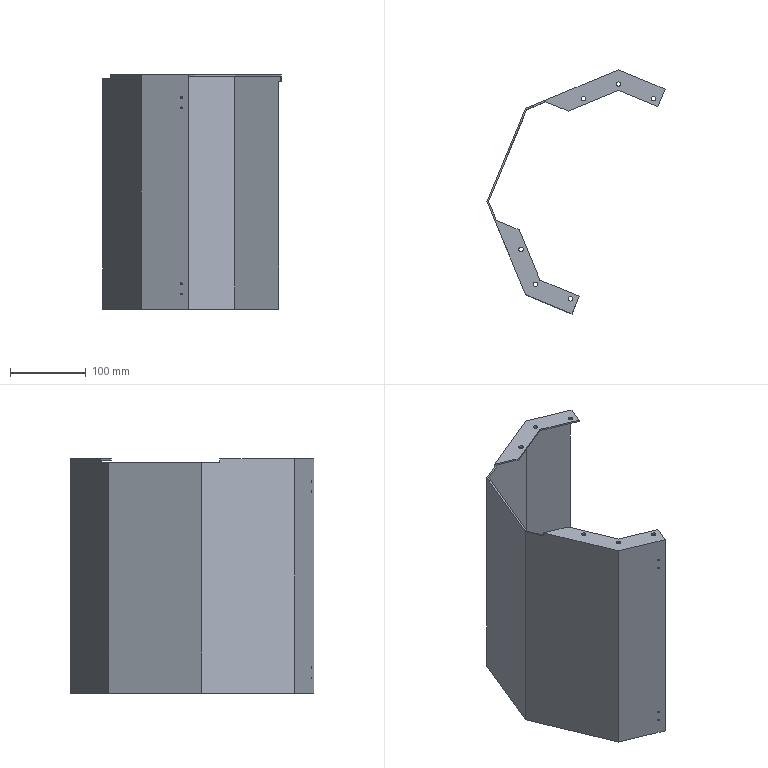Part | SolidWorks | features ICE 5, Cut 1, Extrusion 1, HoleWzd 1, RefAxis 1, Shell 1 | 1 solid | 58 faces | box 235.877 x 323.01 x 310 mm | volume 338319 mm3 | plane 30 | cylinder 28 | commonest cylinder face diameters 6 x20 2.5 x8